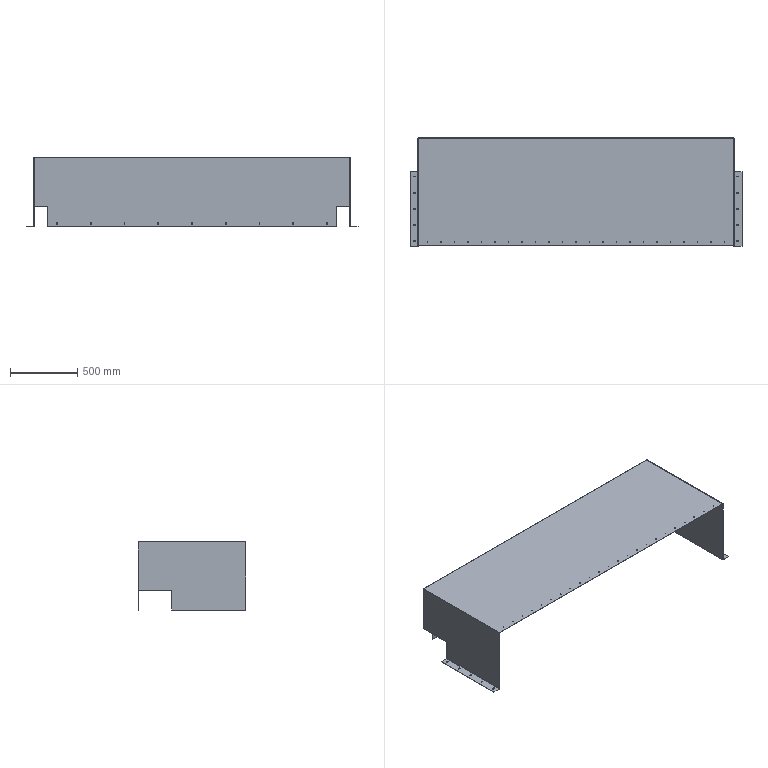Part | SolidWorks | features ICE 4, EdgeFlange 2, LPattern 2, FlatPattern 1, SMBaseFlange 1, SheetMetal 1 | 1 solid | 195 faces | box 2461 x 800 x 510 mm | volume 7657970 mm3 | cylinder 113 | plane 78 | spline 4 | commonest cylinder face diameters 6.5 x57 4.5 x46 1.473 x5 5.473 x5